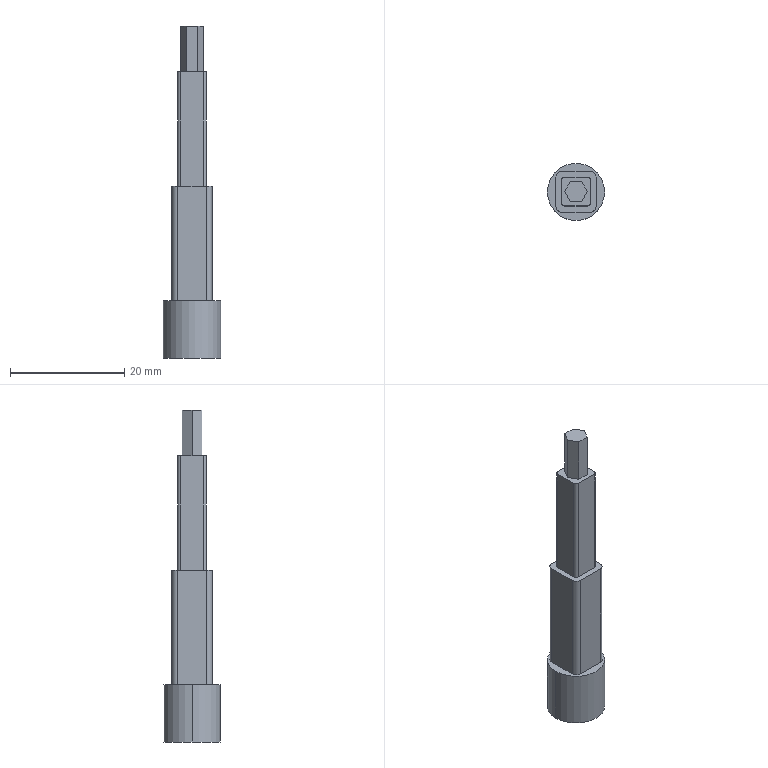Part | SolidWorks | features ICE 3, Fillet 2, Extrusion 1 | 1 solid | 29 faces | box 10 x 10 x 58 mm | volume 2347 mm3 | plane 19 | cylinder 10 | commonest cylinder face diameters 1 x4 2 x4 10 x2
STEP:
#1=CARTESIAN_POINT('',(5.,0.,10.));
#2=VERTEX_POINT('',#1);
#3=CARTESIAN_POINT('',(-5.,0.,10.));
#4=VERTEX_POINT('',#3);
#5=CARTESIAN_POINT('',(0.,0.,10.));
#6=DIRECTION('',(0.,0.,1.));
#7=DIRECTION('',(1.,0.,0.));
#8=AXIS2_PLACEMENT_3D('',#5,#6,#7);
#9=CIRCLE('',#8,5.);
#10=EDGE_CURVE('',#2,#4,#9,.T.);
#11=ORIENTED_EDGE('',*,*,#10,.F.);
#12=CARTESIAN_POINT('',(5.,0.,0.));
#13=VERTEX_POINT('',#12);
#14=CARTESIAN_POINT('',(5.,0.,10.));
#15=DIRECTION('',(0.,0.,-1.));
#16=VECTOR('',#15,1000.);
#17=LINE('',#14,#16);
#18=EDGE_CURVE('',#2,#13,#17,.T.);
#19=ORIENTED_EDGE('',*,*,#18,.T.);
#20=CARTESIAN_POINT('',(-5.,0.,0.));
#21=VERTEX_POINT('',#20);
#22=CARTESIAN_POINT('',(0.,0.,0.));
#23=DIRECTION('',(0.,0.,1.));
#24=DIRECTION('',(1.,0.,0.));
#25=AXIS2_PLACEMENT_3D('',#22,#23,#24);
#26=CIRCLE('',#25,5.);
#27=EDGE_CURVE('',#13,#21,#26,.T.);
#28=ORIENTED_EDGE('',*,*,#27,.T.);
#29=CARTESIAN_POINT('',(-5.,0.,10.));
#30=DIRECTION('',(0.,0.,-1.));
#31=VECTOR('',#30,1000.);
#32=LINE('',#29,#31);
#33=EDGE_CURVE('',#4,#21,#32,.T.);
#34=ORIENTED_EDGE('',*,*,#33,.F.);
#35=EDGE_LOOP('',(#11,#19,#28,#34));
#36=FACE_OUTER_BOUND('',#35,.T.);
#37=CARTESIAN_POINT('',(0.,0.,10.));
#38=DIRECTION('',(0.,0.,-1.));
#39=DIRECTION('',(-1.,0.,0.));
#40=AXIS2_PLACEMENT_3D('',#37,#38,#39);
#41=CYLINDRICAL_SURFACE('',#40,5.);
#42=ADVANCED_FACE('',(#36),#41,.T.);
#43=CARTESIAN_POINT('',(0.,0.,10.));
#44=DIRECTION('',(0.,0.,1.));
#45=DIRECTION('',(1.,0.,0.));
#46=AXIS2_PLACEMENT_3D('',#43,#44,#45);
#47=CIRCLE('',#46,5.);
#48=EDGE_CURVE('',#4,#2,#47,.T.);
#49=ORIENTED_EDGE('',*,*,#48,.T.);
#50=ORIENTED_EDGE('',*,*,#10,.T.);
#51=EDGE_LOOP('',(#49,#50));
#52=FACE_OUTER_BOUND('',#51,.T.);
#53=CARTESIAN_POINT('',(3.5,-2.571,10.));
#54=VERTEX_POINT('',#53);
#55=CARTESIAN_POINT('',(3.5,2.571,10.));
#56=VERTEX_POINT('',#55);
#57=CARTESIAN_POINT('',(3.5,3.571,10.));
#58=DIRECTION('',(0.,1.,0.));
#59=VECTOR('',#58,1000.);
#60=LINE('',#57,#59);
#61=EDGE_CURVE('',#54,#56,#60,.T.);
#62=ORIENTED_EDGE('',*,*,#61,.F.);
#63=CARTESIAN_POINT('',(2.5,-3.571,10.));
#64=VERTEX_POINT('',#63);
#65=CARTESIAN_POINT('',(2.5,-2.571,10.));
#66=DIRECTION('',(0.,0.,-1.));
#67=DIRECTION('',(1.,0.,0.));
#68=AXIS2_PLACEMENT_3D('',#65,#66,#67);
#69=CIRCLE('',#68,1.);
#70=EDGE_CURVE('',#54,#64,#69,.T.);
#71=ORIENTED_EDGE('',*,*,#70,.T.);
#72=CARTESIAN_POINT('',(-2.5,-3.571,10.));
#73=VERTEX_POINT('',#72);
#74=CARTESIAN_POINT('',(-3.5,-3.571,10.));
#75=DIRECTION('',(1.,0.,0.));
#76=VECTOR('',#75,1000.);
#77=LINE('',#74,#76);
#78=EDGE_CURVE('',#73,#64,#77,.T.);
#79=ORIENTED_EDGE('',*,*,#78,.F.);
#80=CARTESIAN_POINT('',(-3.5,-2.571,10.));
#81=VERTEX_POINT('',#80);
#82=CARTESIAN_POINT('',(-2.5,-2.571,10.));
#83=DIRECTION('',(0.,0.,-1.));
#84=DIRECTION('',(1.,0.,0.));
#85=AXIS2_PLACEMENT_3D('',#82,#83,#84);
#86=CIRCLE('',#85,1.);
#87=EDGE_CURVE('',#73,#81,#86,.T.);
#88=ORIENTED_EDGE('',*,*,#87,.T.);
#89=CARTESIAN_POINT('',(-3.5,2.571,10.));
#90=VERTEX_POINT('',#89);
#91=CARTESIAN_POINT('',(-3.5,3.571,10.));
#92=DIRECTION('',(0.,-1.,0.));
#93=VECTOR('',#92,1000.);
#94=LINE('',#91,#93);
#95=EDGE_CURVE('',#90,#81,#94,.T.);
#96=ORIENTED_EDGE('',*,*,#95,.F.);
#97=CARTESIAN_POINT('',(-2.5,3.571,10.));
#98=VERTEX_POINT('',#97);
#99=CARTESIAN_POINT('',(-2.5,2.571,10.));
#100=DIRECTION('',(0.,0.,-1.));
#101=DIRECTION('',(1.,0.,0.));
#102=AXIS2_PLACEMENT_3D('',#99,#100,#101);
#103=CIRCLE('',#102,1.);
#104=EDGE_CURVE('',#90,#98,#103,.T.);
#105=ORIENTED_EDGE('',*,*,#104,.T.);
#106=CARTESIAN_POINT('',(2.5,3.571,10.));
#107=VERTEX_POINT('',#106);
#108=CARTESIAN_POINT('',(-3.5,3.571,10.));
#109=DIRECTION('',(-1.,0.,0.));
#110=VECTOR('',#109,1000.);
#111=LINE('',#108,#110);
#112=EDGE_CURVE('',#107,#98,#111,.T.);
#113=ORIENTED_EDGE('',*,*,#112,.F.);
#114=CARTESIAN_POINT('',(2.5,2.571,10.));
#115=DIRECTION('',(0.,0.,-1.));
#116=DIRECTION('',(1.,0.,0.));
#117=AXIS2_PLACEMENT_3D('',#114,#115,#116);
#118=CIRCLE('',#117,1.);
#119=EDGE_CURVE('',#107,#56,#118,.T.);
#120=ORIENTED_EDGE('',*,*,#119,.T.);
#121=EDGE_LOOP('',(#62,#71,#79,#88,#96,#105,#113,#120));
#122=FACE_BOUND('',#121,.T.);
#123=CARTESIAN_POINT('',(0.,0.,10.));
#124=DIRECTION('',(0.,0.,1.));
#125=DIRECTION('',(1.,0.,0.));
#126=AXIS2_PLACEMENT_3D('',#123,#124,#125);
#127=PLANE('',#126);
#128=ADVANCED_FACE('',(#52,#122),#127,.T.);
#129=ORIENTED_EDGE('',*,*,#18,.F.);
#130=ORIENTED_EDGE('',*,*,#48,.F.);
#131=ORIENTED_EDGE('',*,*,#33,.T.);
#132=CARTESIAN_POINT('',(0.,0.,0.));
#133=DIRECTION('',(0.,0.,1.));
#134=DIRECTION('',(1.,0.,0.));
#135=AXIS2_PLACEMENT_3D('',#132,#133,#134);
#136=CIRCLE('',#135,5.);
#137=EDGE_CURVE('',#21,#13,#136,.T.);
#138=ORIENTED_EDGE('',*,*,#137,.T.);
#139=EDGE_LOOP('',(#129,#130,#131,#138));
#140=FACE_OUTER_BOUND('',#139,.T.);
#141=CARTESIAN_POINT('',(0.,0.,10.));
#142=DIRECTION('',(0.,0.,-1.));
#143=DIRECTION('',(-1.,0.,0.));
#144=AXIS2_PLACEMENT_3D('',#141,#142,#143);
#145=CYLINDRICAL_SURFACE('',#144,5.);
#146=ADVANCED_FACE('',(#140),#145,.T.);
#147=ORIENTED_EDGE('',*,*,#137,.F.);
#148=ORIENTED_EDGE('',*,*,#27,.F.);
#149=EDGE_LOOP('',(#147,#148));
#150=FACE_OUTER_BOUND('',#149,.T.);
#151=CARTESIAN_POINT('',(0.,0.,0.));
#152=DIRECTION('',(0.,0.,1.));
#153=DIRECTION('',(1.,0.,0.));
#154=AXIS2_PLACEMENT_3D('',#151,#152,#153);
#155=PLANE('',#154);
#156=ADVANCED_FACE('',(#150),#155,.F.);
#157=ORIENTED_EDGE('',*,*,#95,.T.);
#158=CARTESIAN_POINT('',(-3.5,-2.571,30.));
#159=VERTEX_POINT('',#158);
#160=CARTESIAN_POINT('',(-3.5,-2.571,30.));
#161=DIRECTION('',(0.,0.,1.));
#162=VECTOR('',#161,1000.);
#163=LINE('',#160,#162);
#164=EDGE_CURVE('',#81,#159,#163,.T.);
#165=ORIENTED_EDGE('',*,*,#164,.T.);
#166=CARTESIAN_POINT('',(-3.5,2.571,30.));
#167=VERTEX_POINT('',#166);
#168=CARTESIAN_POINT('',(-3.5,3.571,30.));
#169=DIRECTION('',(0.,-1.,0.));
#170=VECTOR('',#169,1000.);
#171=LINE('',#168,#170);
#172=EDGE_CURVE('',#167,#159,#171,.T.);
#173=ORIENTED_EDGE('',*,*,#172,.F.);
#174=CARTESIAN_POINT('',(-3.5,2.571,30.));
#175=DIRECTION('',(0.,0.,-1.));
#176=VECTOR('',#175,1000.);
#177=LINE('',#174,#176);
#178=EDGE_CURVE('',#167,#90,#177,.T.);
#179=ORIENTED_EDGE('',*,*,#178,.T.);
#180=EDGE_LOOP('',(#157,#165,#173,#179));
#181=FACE_OUTER_BOUND('',#180,.T.);
#182=CARTESIAN_POINT('',(-3.5,3.571,30.));
#183=DIRECTION('',(1.,0.,0.));
#184=DIRECTION('',(0.,0.,-1.));
#185=AXIS2_PLACEMENT_3D('',#182,#183,#184);
#186=PLANE('',#185);
#187=ADVANCED_FACE('',(#181),#186,.F.);
#188=ORIENTED_EDGE('',*,*,#78,.T.);
#189=CARTESIAN_POINT('',(2.5,-3.571,30.));
#190=VERTEX_POINT('',#189);
#191=CARTESIAN_POINT('',(2.5,-3.571,30.));
#192=DIRECTION('',(0.,0.,1.));
#193=VECTOR('',#192,1000.);
#194=LINE('',#191,#193);
#195=EDGE_CURVE('',#64,#190,#194,.T.);
#196=ORIENTED_EDGE('',*,*,#195,.T.);
#197=CARTESIAN_POINT('',(-2.5,-3.571,30.));
#198=VERTEX_POINT('',#197);
#199=CARTESIAN_POINT('',(-3.5,-3.571,30.));
#200=DIRECTION('',(1.,0.,0.));
#201=VECTOR('',#200,1000.);
#202=LINE('',#199,#201);
#203=EDGE_CURVE('',#198,#190,#202,.T.);
#204=ORIENTED_EDGE('',*,*,#203,.F.);
#205=CARTESIAN_POINT('',(-2.5,-3.571,30.));
#206=DIRECTION('',(0.,0.,-1.));
#207=VECTOR('',#206,1000.);
#208=LINE('',#205,#207);
#209=EDGE_CURVE('',#198,#73,#208,.T.);
#210=ORIENTED_EDGE('',*,*,#209,.T.);
#211=EDGE_LOOP('',(#188,#196,#204,#210));
#212=FACE_OUTER_BOUND('',#211,.T.);
#213=CARTESIAN_POINT('',(-3.5,-3.571,30.));
#214=DIRECTION('',(0.,1.,0.));
#215=DIRECTION('',(0.,0.,1.));
#216=AXIS2_PLACEMENT_3D('',#213,#214,#215);
#217=PLANE('',#216);
#218=ADVANCED_FACE('',(#212),#217,.F.);
#219=CARTESIAN_POINT('',(3.5,-2.571,30.));
#220=VERTEX_POINT('',#219);
#221=CARTESIAN_POINT('',(3.5,2.571,30.));
#222=VERTEX_POINT('',#221);
#223=CARTESIAN_POINT('',(3.5,3.571,30.));
#224=DIRECTION('',(0.,1.,0.));
#225=VECTOR('',#224,1000.);
#226=LINE('',#223,#225);
#227=EDGE_CURVE('',#220,#222,#226,.T.);
#228=ORIENTED_EDGE('',*,*,#227,.F.);
#229=CARTESIAN_POINT('',(3.5,-2.571,30.));
#230=DIRECTION('',(0.,0.,-1.));
#231=VECTOR('',#230,1000.);
#232=LINE('',#229,#231);
#233=EDGE_CURVE('',#220,#54,#232,.T.);
#234=ORIENTED_EDGE('',*,*,#233,.T.);
#235=ORIENTED_EDGE('',*,*,#61,.T.);
#236=CARTESIAN_POINT('',(3.5,2.571,30.));
#237=DIRECTION('',(0.,0.,1.));
#238=VECTOR('',#237,1000.);
#239=LINE('',#236,#238);
#240=EDGE_CURVE('',#56,#222,#239,.T.);
#241=ORIENTED_EDGE('',*,*,#240,.T.);
#242=EDGE_LOOP('',(#228,#234,#235,#241));
#243=FACE_OUTER_BOUND('',#242,.T.);
#244=CARTESIAN_POINT('',(3.5,3.571,30.));
#245=DIRECTION('',(-1.,0.,0.));
#246=DIRECTION('',(0.,0.,1.));
#247=AXIS2_PLACEMENT_3D('',#244,#245,#246);
#248=PLANE('',#247);
#249=ADVANCED_FACE('',(#243),#248,.F.);
#250=ORIENTED_EDGE('',*,*,#112,.T.);
#251=CARTESIAN_POINT('',(-2.5,3.571,30.));
#252=VERTEX_POINT('',#251);
#253=CARTESIAN_POINT('',(-2.5,3.571,30.));
#254=DIRECTION('',(0.,0.,1.));
#255=VECTOR('',#254,1000.);
#256=LINE('',#253,#255);
#257=EDGE_CURVE('',#98,#252,#256,.T.);
#258=ORIENTED_EDGE('',*,*,#257,.T.);
#259=CARTESIAN_POINT('',(2.5,3.571,30.));
#260=VERTEX_POINT('',#259);
#261=CARTESIAN_POINT('',(-3.5,3.571,30.));
#262=DIRECTION('',(-1.,0.,0.));
#263=VECTOR('',#262,1000.);
#264=LINE('',#261,#263);
#265=EDGE_CURVE('',#260,#252,#264,.T.);
#266=ORIENTED_EDGE('',*,*,#265,.F.);
#267=CARTESIAN_POINT('',(2.5,3.571,30.));
#268=DIRECTION('',(0.,0.,-1.));
#269=VECTOR('',#268,1000.);
#270=LINE('',#267,#269);
#271=EDGE_CURVE('',#260,#107,#270,.T.);
#272=ORIENTED_EDGE('',*,*,#271,.T.);
#273=EDGE_LOOP('',(#250,#258,#266,#272));
#274=FACE_OUTER_BOUND('',#273,.T.);
#275=CARTESIAN_POINT('',(-3.5,3.571,30.));
#276=DIRECTION('',(0.,-1.,0.));
#277=DIRECTION('',(0.,0.,-1.));
#278=AXIS2_PLACEMENT_3D('',#275,#276,#277);
#279=PLANE('',#278);
#280=ADVANCED_FACE('',(#274),#279,.F.);
#281=CARTESIAN_POINT('',(-2.5,2.,30.));
#282=VERTEX_POINT('',#281);
#283=CARTESIAN_POINT('',(-2.5,-2.,30.));
#284=VERTEX_POINT('',#283);
#285=CARTESIAN_POINT('',(-2.5,-2.5,30.));
#286=DIRECTION('',(0.,-1.,0.));
#287=VECTOR('',#286,1000.);
#288=LINE('',#285,#287);
#289=EDGE_CURVE('',#282,#284,#288,.T.);
#290=ORIENTED_EDGE('',*,*,#289,.F.);
#291=CARTESIAN_POINT('',(-2.,2.5,30.));
#292=VERTEX_POINT('',#291);
#293=CARTESIAN_POINT('',(-2.,2.,30.));
#294=DIRECTION('',(0.,0.,-1.));
#295=DIRECTION('',(1.,0.,0.));
#296=AXIS2_PLACEMENT_3D('',#293,#294,#295);
#297=CIRCLE('',#296,0.5);
#298=EDGE_CURVE('',#282,#292,#297,.T.);
#299=ORIENTED_EDGE('',*,*,#298,.T.);
#300=CARTESIAN_POINT('',(2.,2.5,30.));
#301=VERTEX_POINT('',#300);
#302=CARTESIAN_POINT('',(2.5,2.5,30.));
#303=DIRECTION('',(-1.,0.,0.));
#304=VECTOR('',#303,1000.);
#305=LINE('',#302,#304);
#306=EDGE_CURVE('',#301,#292,#305,.T.);
#307=ORIENTED_EDGE('',*,*,#306,.F.);
#308=CARTESIAN_POINT('',(2.5,2.,30.));
#309=VERTEX_POINT('',#308);
#310=CARTESIAN_POINT('',(2.,2.,30.));
#311=DIRECTION('',(0.,0.,-1.));
#312=DIRECTION('',(1.,0.,0.));
#313=AXIS2_PLACEMENT_3D('',#310,#311,#312);
#314=CIRCLE('',#313,0.5);
#315=EDGE_CURVE('',#301,#309,#314,.T.);
#316=ORIENTED_EDGE('',*,*,#315,.T.);
#317=CARTESIAN_POINT('',(2.5,-2.,30.));
#318=VERTEX_POINT('',#317);
#319=CARTESIAN_POINT('',(2.5,-2.5,30.));
#320=DIRECTION('',(0.,1.,0.));
#321=VECTOR('',#320,1000.);
#322=LINE('',#319,#321);
#323=EDGE_CURVE('',#318,#309,#322,.T.);
#324=ORIENTED_EDGE('',*,*,#323,.F.);
#325=CARTESIAN_POINT('',(2.,-2.5,30.));
#326=VERTEX_POINT('',#325);
#327=CARTESIAN_POINT('',(2.,-2.,30.));
#328=DIRECTION('',(0.,0.,-1.));
#329=DIRECTION('',(1.,0.,0.));
#330=AXIS2_PLACEMENT_3D('',#327,#328,#329);
#331=CIRCLE('',#330,0.5);
#332=EDGE_CURVE('',#318,#326,#331,.T.);
#333=ORIENTED_EDGE('',*,*,#332,.T.);
#334=CARTESIAN_POINT('',(-2.,-2.5,30.));
#335=VERTEX_POINT('',#334);
#336=CARTESIAN_POINT('',(2.5,-2.5,30.));
#337=DIRECTION('',(1.,0.,0.));
#338=VECTOR('',#337,1000.);
#339=LINE('',#336,#338);
#340=EDGE_CURVE('',#335,#326,#339,.T.);
#341=ORIENTED_EDGE('',*,*,#340,.F.);
#342=CARTESIAN_POINT('',(-2.,-2.,30.));
#343=DIRECTION('',(0.,0.,-1.));
#344=DIRECTION('',(1.,0.,0.));
#345=AXIS2_PLACEMENT_3D('',#342,#343,#344);
#346=CIRCLE('',#345,0.5);
#347=EDGE_CURVE('',#335,#284,#346,.T.);
#348=ORIENTED_EDGE('',*,*,#347,.T.);
#349=EDGE_LOOP('',(#290,#299,#307,#316,#324,#333,#341,#348));
#350=FACE_BOUND('',#349,.T.);
#351=ORIENTED_EDGE('',*,*,#203,.T.);
#352=CARTESIAN_POINT('',(2.5,-2.571,30.));
#353=DIRECTION('',(0.,0.,1.));
#354=DIRECTION('',(1.,0.,0.));
#355=AXIS2_PLACEMENT_3D('',#352,#353,#354);
#356=CIRCLE('',#355,1.);
#357=EDGE_CURVE('',#190,#220,#356,.T.);
#358=ORIENTED_EDGE('',*,*,#357,.T.);
#359=ORIENTED_EDGE('',*,*,#227,.T.);
#360=CARTESIAN_POINT('',(2.5,2.571,30.));
#361=DIRECTION('',(0.,0.,1.));
#362=DIRECTION('',(1.,0.,0.));
#363=AXIS2_PLACEMENT_3D('',#360,#361,#362);
#364=CIRCLE('',#363,1.);
#365=EDGE_CURVE('',#222,#260,#364,.T.);
#366=ORIENTED_EDGE('',*,*,#365,.T.);
#367=ORIENTED_EDGE('',*,*,#265,.T.);
#368=CARTESIAN_POINT('',(-2.5,2.571,30.));
#369=DIRECTION('',(0.,0.,1.));
#370=DIRECTION('',(1.,0.,0.));
#371=AXIS2_PLACEMENT_3D('',#368,#369,#370);
#372=CIRCLE('',#371,1.);
#373=EDGE_CURVE('',#252,#167,#372,.T.);
#374=ORIENTED_EDGE('',*,*,#373,.T.);
#375=ORIENTED_EDGE('',*,*,#172,.T.);
#376=CARTESIAN_POINT('',(-2.5,-2.571,30.));
#377=DIRECTION('',(0.,0.,1.));
#378=DIRECTION('',(1.,0.,0.));
#379=AXIS2_PLACEMENT_3D('',#376,#377,#378);
#380=CIRCLE('',#379,1.);
#381=EDGE_CURVE('',#159,#198,#380,.T.);
#382=ORIENTED_EDGE('',*,*,#381,.T.);
#383=EDGE_LOOP('',(#351,#358,#359,#366,#367,#374,#375,#382));
#384=FACE_OUTER_BOUND('',#383,.T.);
#385=CARTESIAN_POINT('',(0.,0.,30.));
#386=DIRECTION('',(0.,0.,1.));
#387=DIRECTION('',(1.,0.,0.));
#388=AXIS2_PLACEMENT_3D('',#385,#386,#387);
#389=PLANE('',#388);
#390=ADVANCED_FACE('',(#350,#384),#389,.T.);
#391=ORIENTED_EDGE('',*,*,#357,.F.);
#392=ORIENTED_EDGE('',*,*,#195,.F.);
#393=ORIENTED_EDGE('',*,*,#70,.F.);
#394=ORIENTED_EDGE('',*,*,#233,.F.);
#395=EDGE_LOOP('',(#391,#392,#393,#394));
#396=FACE_OUTER_BOUND('',#395,.T.);
#397=CARTESIAN_POINT('',(2.5,-2.571,30.));
#398=DIRECTION('',(0.,0.,-1.));
#399=DIRECTION('',(-1.,0.,0.));
#400=AXIS2_PLACEMENT_3D('',#397,#398,#399);
#401=CYLINDRICAL_SURFACE('',#400,1.);
#402=ADVANCED_FACE('',(#396),#401,.T.);
#403=ORIENTED_EDGE('',*,*,#381,.F.);
#404=ORIENTED_EDGE('',*,*,#164,.F.);
#405=ORIENTED_EDGE('',*,*,#87,.F.);
#406=ORIENTED_EDGE('',*,*,#209,.F.);
#407=EDGE_LOOP('',(#403,#404,#405,#406));
#408=FACE_OUTER_BOUND('',#407,.T.);
#409=CARTESIAN_POINT('',(-2.5,-2.571,30.));
#410=DIRECTION('',(0.,0.,-1.));
#411=DIRECTION('',(-1.,0.,0.));
#412=AXIS2_PLACEMENT_3D('',#409,#410,#411);
#413=CYLINDRICAL_SURFACE('',#412,1.);
#414=ADVANCED_FACE('',(#408),#413,.T.);
#415=ORIENTED_EDGE('',*,*,#373,.F.);
#416=ORIENTED_EDGE('',*,*,#257,.F.);
#417=ORIENTED_EDGE('',*,*,#104,.F.);
#418=ORIENTED_EDGE('',*,*,#178,.F.);
#419=EDGE_LOOP('',(#415,#416,#417,#418));
#420=FACE_OUTER_BOUND('',#419,.T.);
#421=CARTESIAN_POINT('',(-2.5,2.571,30.));
#422=DIRECTION('',(0.,0.,-1.));
#423=DIRECTION('',(-1.,0.,0.));
#424=AXIS2_PLACEMENT_3D('',#421,#422,#423);
#425=CYLINDRICAL_SURFACE('',#424,1.);
#426=ADVANCED_FACE('',(#420),#425,.T.);
#427=ORIENTED_EDGE('',*,*,#365,.F.);
#428=ORIENTED_EDGE('',*,*,#240,.F.);
#429=ORIENTED_EDGE('',*,*,#119,.F.);
#430=ORIENTED_EDGE('',*,*,#271,.F.);
#431=EDGE_LOOP('',(#427,#428,#429,#430));
#432=FACE_OUTER_BOUND('',#431,.T.);
#433=CARTESIAN_POINT('',(2.5,2.571,30.));
#434=DIRECTION('',(0.,0.,-1.));
#435=DIRECTION('',(-1.,0.,0.));
#436=AXIS2_PLACEMENT_3D('',#433,#434,#435);
#437=CYLINDRICAL_SURFACE('',#436,1.);
#438=ADVANCED_FACE('',(#432),#437,.T.);
#439=ORIENTED_EDGE('',*,*,#289,.T.);
#440=CARTESIAN_POINT('',(-2.5,-2.,50.));
#441=VERTEX_POINT('',#440);
#442=CARTESIAN_POINT('',(-2.5,-2.,50.));
#443=DIRECTION('',(0.,0.,1.));
#444=VECTOR('',#443,1000.);
#445=LINE('',#442,#444);
#446=EDGE_CURVE('',#284,#441,#445,.T.);
#447=ORIENTED_EDGE('',*,*,#446,.T.);
#448=CARTESIAN_POINT('',(-2.5,2.,50.));
#449=VERTEX_POINT('',#448);
#450=CARTESIAN_POINT('',(-2.5,-2.5,50.));
#451=DIRECTION('',(0.,-1.,0.));
#452=VECTOR('',#451,1000.);
#453=LINE('',#450,#452);
#454=EDGE_CURVE('',#449,#441,#453,.T.);
#455=ORIENTED_EDGE('',*,*,#454,.F.);
#456=CARTESIAN_POINT('',(-2.5,2.,50.));
#457=DIRECTION('',(0.,0.,-1.));
#458=VECTOR('',#457,1000.);
#459=LINE('',#456,#458);
#460=EDGE_CURVE('',#449,#282,#459,.T.);
#461=ORIENTED_EDGE('',*,*,#460,.T.);
#462=EDGE_LOOP('',(#439,#447,#455,#461));
#463=FACE_OUTER_BOUND('',#462,.T.);
#464=CARTESIAN_POINT('',(-2.5,-2.5,50.));
#465=DIRECTION('',(1.,0.,0.));
#466=DIRECTION('',(0.,0.,-1.));
#467=AXIS2_PLACEMENT_3D('',#464,#465,#466);
#468=PLANE('',#467);
#469=ADVANCED_FACE('',(#463),#468,.F.);
#470=ORIENTED_EDGE('',*,*,#340,.T.);
#471=CARTESIAN_POINT('',(2.,-2.5,50.));
#472=VERTEX_POINT('',#471);
#473=CARTESIAN_POINT('',(2.,-2.5,50.));
#474=DIRECTION('',(0.,0.,1.));
#475=VECTOR('',#474,1000.);
#476=LINE('',#473,#475);
#477=EDGE_CURVE('',#326,#472,#476,.T.);
#478=ORIENTED_EDGE('',*,*,#477,.T.);
#479=CARTESIAN_POINT('',(-2.,-2.5,50.));
#480=VERTEX_POINT('',#479);
#481=CARTESIAN_POINT('',(2.5,-2.5,50.));
#482=DIRECTION('',(1.,0.,0.));
#483=VECTOR('',#482,1000.);
#484=LINE('',#481,#483);
#485=EDGE_CURVE('',#480,#472,#484,.T.);
#486=ORIENTED_EDGE('',*,*,#485,.F.);
#487=CARTESIAN_POINT('',(-2.,-2.5,50.));
#488=DIRECTION('',(0.,0.,-1.));
#489=VECTOR('',#488,1000.);
#490=LINE('',#487,#489);
#491=EDGE_CURVE('',#480,#335,#490,.T.);
#492=ORIENTED_EDGE('',*,*,#491,.T.);
#493=EDGE_LOOP('',(#470,#478,#486,#492));
#494=FACE_OUTER_BOUND('',#493,.T.);
#495=CARTESIAN_POINT('',(2.5,-2.5,50.));
#496=DIRECTION('',(0.,1.,0.));
#497=DIRECTION('',(-1.,0.,0.));
#498=AXIS2_PLACEMENT_3D('',#495,#496,#497);
#499=PLANE('',#498);
#500=ADVANCED_FACE('',(#494),#499,.F.);
#501=CARTESIAN_POINT('',(2.5,-2.,50.));
#502=VERTEX_POINT('',#501);
#503=CARTESIAN_POINT('',(2.5,2.,50.));
#504=VERTEX_POINT('',#503);
#505=CARTESIAN_POINT('',(2.5,-2.5,50.));
#506=DIRECTION('',(0.,1.,0.));
#507=VECTOR('',#506,1000.);
#508=LINE('',#505,#507);
#509=EDGE_CURVE('',#502,#504,#508,.T.);
#510=ORIENTED_EDGE('',*,*,#509,.F.);
#511=CARTESIAN_POINT('',(2.5,-2.,50.));
#512=DIRECTION('',(0.,0.,-1.));
#513=VECTOR('',#512,1000.);
#514=LINE('',#511,#513);
#515=EDGE_CURVE('',#502,#318,#514,.T.);
#516=ORIENTED_EDGE('',*,*,#515,.T.);
#517=ORIENTED_EDGE('',*,*,#323,.T.);
#518=CARTESIAN_POINT('',(2.5,2.,50.));
#519=DIRECTION('',(0.,0.,1.));
#520=VECTOR('',#519,1000.);
#521=LINE('',#518,#520);
#522=EDGE_CURVE('',#309,#504,#521,.T.);
#523=ORIENTED_EDGE('',*,*,#522,.T.);
#524=EDGE_LOOP('',(#510,#516,#517,#523));
#525=FACE_OUTER_BOUND('',#524,.T.);
#526=CARTESIAN_POINT('',(2.5,-2.5,50.));
#527=DIRECTION('',(-1.,0.,0.));
#528=DIRECTION('',(0.,0.,1.));
#529=AXIS2_PLACEMENT_3D('',#526,#527,#528);
#530=PLANE('',#529);
#531=ADVANCED_FACE('',(#525),#530,.F.);
#532=ORIENTED_EDGE('',*,*,#306,.T.);
#533=CARTESIAN_POINT('',(-2.,2.5,50.));
#534=VERTEX_POINT('',#533);
#535=CARTESIAN_POINT('',(-2.,2.5,50.));
#536=DIRECTION('',(0.,0.,1.));
#537=VECTOR('',#536,1000.);
#538=LINE('',#535,#537);
#539=EDGE_CURVE('',#292,#534,#538,.T.);
#540=ORIENTED_EDGE('',*,*,#539,.T.);
#541=CARTESIAN_POINT('',(2.,2.5,50.));
#542=VERTEX_POINT('',#541);
#543=CARTESIAN_POINT('',(2.5,2.5,50.));
#544=DIRECTION('',(-1.,0.,0.));
#545=VECTOR('',#544,1000.);
#546=LINE('',#543,#545);
#547=EDGE_CURVE('',#542,#534,#546,.T.);
#548=ORIENTED_EDGE('',*,*,#547,.F.);
#549=CARTESIAN_POINT('',(2.,2.5,50.));
#550=DIRECTION('',(0.,0.,-1.));
#551=VECTOR('',#550,1000.);
#552=LINE('',#549,#551);
#553=EDGE_CURVE('',#542,#301,#552,.T.);
#554=ORIENTED_EDGE('',*,*,#553,.T.);
#555=EDGE_LOOP('',(#532,#540,#548,#554));
#556=FACE_OUTER_BOUND('',#555,.T.);
#557=CARTESIAN_POINT('',(2.5,2.5,50.));
#558=DIRECTION('',(0.,-1.,0.));
#559=DIRECTION('',(0.,0.,-1.));
#560=AXIS2_PLACEMENT_3D('',#557,#558,#559);
#561=PLANE('',#560);
#562=ADVANCED_FACE('',(#556),#561,.F.);
#563=CARTESIAN_POINT('',(2.,0.,50.));
#564=VERTEX_POINT('',#563);
#565=CARTESIAN_POINT('',(1.,1.732,50.));
#566=VERTEX_POINT('',#565);
#567=CARTESIAN_POINT('',(2.,0.,50.));
#568=DIRECTION('',(-0.5,0.866,0.));
#569=VECTOR('',#568,1000.);
#570=LINE('',#567,#569);
#571=EDGE_CURVE('',#564,#566,#570,.T.);
#572=ORIENTED_EDGE('',*,*,#571,.F.);
#573=CARTESIAN_POINT('',(1.,-1.732,50.));
#574=VERTEX_POINT('',#573);
#575=CARTESIAN_POINT('',(1.,-1.732,50.));
#576=DIRECTION('',(0.5,0.866,0.));
#577=VECTOR('',#576,1000.);
#578=LINE('',#575,#577);
#579=EDGE_CURVE('',#574,#564,#578,.T.);
#580=ORIENTED_EDGE('',*,*,#579,.F.);
#581=CARTESIAN_POINT('',(-1.,-1.732,50.));
#582=VERTEX_POINT('',#581);
#583=CARTESIAN_POINT('',(-1.,-1.732,50.));
#584=DIRECTION('',(1.,0.,0.));
#585=VECTOR('',#584,1000.);
#586=LINE('',#583,#585);
#587=EDGE_CURVE('',#582,#574,#586,.T.);
#588=ORIENTED_EDGE('',*,*,#587,.F.);
#589=CARTESIAN_POINT('',(-2.,0.,50.));
#590=VERTEX_POINT('',#589);
#591=CARTESIAN_POINT('',(-2.,0.,50.));
#592=DIRECTION('',(0.5,-0.866,0.));
#593=VECTOR('',#592,1000.);
#594=LINE('',#591,#593);
#595=EDGE_CURVE('',#590,#582,#594,.T.);
#596=ORIENTED_EDGE('',*,*,#595,.F.);
#597=CARTESIAN_POINT('',(-1.,1.732,50.));
#598=VERTEX_POINT('',#597);
#599=CARTESIAN_POINT('',(-1.,1.732,50.));
#600=DIRECTION('',(-0.5,-0.866,0.));
#601=VECTOR('',#600,1000.);
#602=LINE('',#599,#601);
#603=EDGE_CURVE('',#598,#590,#602,.T.);
#604=ORIENTED_EDGE('',*,*,#603,.F.);
#605=CARTESIAN_POINT('',(1.,1.732,50.));
#606=DIRECTION('',(-1.,0.,0.));
#607=VECTOR('',#606,1000.);
#608=LINE('',#605,#607);
#609=EDGE_CURVE('',#566,#598,#608,.T.);
#610=ORIENTED_EDGE('',*,*,#609,.F.);
#611=EDGE_LOOP('',(#572,#580,#588,#596,#604,#610));
#612=FACE_BOUND('',#611,.T.);
#613=ORIENTED_EDGE('',*,*,#485,.T.);
#614=CARTESIAN_POINT('',(2.,-2.,50.));
#615=DIRECTION('',(0.,0.,1.));
#616=DIRECTION('',(1.,0.,0.));
#617=AXIS2_PLACEMENT_3D('',#614,#615,#616);
#618=CIRCLE('',#617,0.5);
#619=EDGE_CURVE('',#472,#502,#618,.T.);
#620=ORIENTED_EDGE('',*,*,#619,.T.);
#621=ORIENTED_EDGE('',*,*,#509,.T.);
#622=CARTESIAN_POINT('',(2.,2.,50.));
#623=DIRECTION('',(0.,0.,1.));
#624=DIRECTION('',(1.,0.,0.));
#625=AXIS2_PLACEMENT_3D('',#622,#623,#624);
#626=CIRCLE('',#625,0.5);
#627=EDGE_CURVE('',#504,#542,#626,.T.);
#628=ORIENTED_EDGE('',*,*,#627,.T.);
#629=ORIENTED_EDGE('',*,*,#547,.T.);
#630=CARTESIAN_POINT('',(-2.,2.,50.));
#631=DIRECTION('',(0.,0.,1.));
#632=DIRECTION('',(1.,0.,0.));
#633=AXIS2_PLACEMENT_3D('',#630,#631,#632);
#634=CIRCLE('',#633,0.5);
#635=EDGE_CURVE('',#534,#449,#634,.T.);
#636=ORIENTED_EDGE('',*,*,#635,.T.);
#637=ORIENTED_EDGE('',*,*,#454,.T.);
#638=CARTESIAN_POINT('',(-2.,-2.,50.));
#639=DIRECTION('',(0.,0.,1.));
#640=DIRECTION('',(1.,0.,0.));
#641=AXIS2_PLACEMENT_3D('',#638,#639,#640);
#642=CIRCLE('',#641,0.5);
#643=EDGE_CURVE('',#441,#480,#642,.T.);
#644=ORIENTED_EDGE('',*,*,#643,.T.);
#645=EDGE_LOOP('',(#613,#620,#621,#628,#629,#636,#637,#644));
#646=FACE_OUTER_BOUND('',#645,.T.);
#647=CARTESIAN_POINT('',(0.,0.,50.));
#648=DIRECTION('',(0.,0.,1.));
#649=DIRECTION('',(1.,0.,0.));
#650=AXIS2_PLACEMENT_3D('',#647,#648,#649);
#651=PLANE('',#650);
#652=ADVANCED_FACE('',(#612,#646),#651,.T.);
#653=ORIENTED_EDGE('',*,*,#619,.F.);
#654=ORIENTED_EDGE('',*,*,#477,.F.);
#655=ORIENTED_EDGE('',*,*,#332,.F.);
#656=ORIENTED_EDGE('',*,*,#515,.F.);
#657=EDGE_LOOP('',(#653,#654,#655,#656));
#658=FACE_OUTER_BOUND('',#657,.T.);
#659=CARTESIAN_POINT('',(2.,-2.,50.));
#660=DIRECTION('',(0.,0.,-1.));
#661=DIRECTION('',(-1.,0.,0.));
#662=AXIS2_PLACEMENT_3D('',#659,#660,#661);
#663=CYLINDRICAL_SURFACE('',#662,0.5);
#664=ADVANCED_FACE('',(#658),#663,.T.);
#665=ORIENTED_EDGE('',*,*,#643,.F.);
#666=ORIENTED_EDGE('',*,*,#446,.F.);
#667=ORIENTED_EDGE('',*,*,#347,.F.);
#668=ORIENTED_EDGE('',*,*,#491,.F.);
#669=EDGE_LOOP('',(#665,#666,#667,#668));
#670=FACE_OUTER_BOUND('',#669,.T.);
#671=CARTESIAN_POINT('',(-2.,-2.,50.));
#672=DIRECTION('',(0.,0.,-1.));
#673=DIRECTION('',(-1.,0.,0.));
#674=AXIS2_PLACEMENT_3D('',#671,#672,#673);
#675=CYLINDRICAL_SURFACE('',#674,0.5);
#676=ADVANCED_FACE('',(#670),#675,.T.);
#677=ORIENTED_EDGE('',*,*,#635,.F.);
#678=ORIENTED_EDGE('',*,*,#539,.F.);
#679=ORIENTED_EDGE('',*,*,#298,.F.);
#680=ORIENTED_EDGE('',*,*,#460,.F.);
#681=EDGE_LOOP('',(#677,#678,#679,#680));
#682=FACE_OUTER_BOUND('',#681,.T.);
#683=CARTESIAN_POINT('',(-2.,2.,50.));
#684=DIRECTION('',(0.,0.,-1.));
#685=DIRECTION('',(-1.,0.,0.));
#686=AXIS2_PLACEMENT_3D('',#683,#684,#685);
#687=CYLINDRICAL_SURFACE('',#686,0.5);
#688=ADVANCED_FACE('',(#682),#687,.T.);
#689=ORIENTED_EDGE('',*,*,#627,.F.);
#690=ORIENTED_EDGE('',*,*,#522,.F.);
#691=ORIENTED_EDGE('',*,*,#315,.F.);
#692=ORIENTED_EDGE('',*,*,#553,.F.);
#693=EDGE_LOOP('',(#689,#690,#691,#692));
#694=FACE_OUTER_BOUND('',#693,.T.);
#695=CARTESIAN_POINT('',(2.,2.,50.));
#696=DIRECTION('',(0.,0.,-1.));
#697=DIRECTION('',(-1.,0.,0.));
#698=AXIS2_PLACEMENT_3D('',#695,#696,#697);
#699=CYLINDRICAL_SURFACE('',#698,0.5);
#700=ADVANCED_FACE('',(#694),#699,.T.);
#701=ORIENTED_EDGE('',*,*,#571,.T.);
#702=CARTESIAN_POINT('',(1.,1.732,58.));
#703=VERTEX_POINT('',#702);
#704=CARTESIAN_POINT('',(1.,1.732,58.));
#705=DIRECTION('',(0.,0.,-1.));
#706=VECTOR('',#705,1000.);
#707=LINE('',#704,#706);
#708=EDGE_CURVE('',#703,#566,#707,.T.);
#709=ORIENTED_EDGE('',*,*,#708,.F.);
#710=CARTESIAN_POINT('',(2.,0.,58.));
#711=VERTEX_POINT('',#710);
#712=CARTESIAN_POINT('',(2.,0.,58.));
#713=DIRECTION('',(-0.5,0.866,0.));
#714=VECTOR('',#713,1000.);
#715=LINE('',#712,#714);
#716=EDGE_CURVE('',#711,#703,#715,.T.);
#717=ORIENTED_EDGE('',*,*,#716,.F.);
#718=CARTESIAN_POINT('',(2.,0.,58.));
#719=DIRECTION('',(0.,0.,-1.));
#720=VECTOR('',#719,1000.);
#721=LINE('',#718,#720);
#722=EDGE_CURVE('',#711,#564,#721,.T.);
#723=ORIENTED_EDGE('',*,*,#722,.T.);
#724=EDGE_LOOP('',(#701,#709,#717,#723));
#725=FACE_OUTER_BOUND('',#724,.T.);
#726=CARTESIAN_POINT('',(2.,0.,58.));
#727=DIRECTION('',(-0.866,-0.5,0.));
#728=DIRECTION('',(0.5,-0.866,0.));
#729=AXIS2_PLACEMENT_3D('',#726,#727,#728);
#730=PLANE('',#729);
#731=ADVANCED_FACE('',(#725),#730,.F.);
#732=ORIENTED_EDGE('',*,*,#609,.T.);
#733=CARTESIAN_POINT('',(-1.,1.732,58.));
#734=VERTEX_POINT('',#733);
#735=CARTESIAN_POINT('',(-1.,1.732,58.));
#736=DIRECTION('',(0.,0.,-1.));
#737=VECTOR('',#736,1000.);
#738=LINE('',#735,#737);
#739=EDGE_CURVE('',#734,#598,#738,.T.);
#740=ORIENTED_EDGE('',*,*,#739,.F.);
#741=CARTESIAN_POINT('',(1.,1.732,58.));
#742=DIRECTION('',(-1.,0.,0.));
#743=VECTOR('',#742,1000.);
#744=LINE('',#741,#743);
#745=EDGE_CURVE('',#703,#734,#744,.T.);
#746=ORIENTED_EDGE('',*,*,#745,.F.);
#747=ORIENTED_EDGE('',*,*,#708,.T.);
#748=EDGE_LOOP('',(#732,#740,#746,#747));
#749=FACE_OUTER_BOUND('',#748,.T.);
#750=CARTESIAN_POINT('',(1.,1.732,58.));
#751=DIRECTION('',(0.,-1.,0.));
#752=DIRECTION('',(1.,0.,0.));
#753=AXIS2_PLACEMENT_3D('',#750,#751,#752);
#754=PLANE('',#753);
#755=ADVANCED_FACE('',(#749),#754,.F.);
#756=ORIENTED_EDGE('',*,*,#603,.T.);
#757=CARTESIAN_POINT('',(-2.,0.,58.));
#758=VERTEX_POINT('',#757);
#759=CARTESIAN_POINT('',(-2.,0.,58.));
#760=DIRECTION('',(0.,0.,-1.));
#761=VECTOR('',#760,1000.);
#762=LINE('',#759,#761);
#763=EDGE_CURVE('',#758,#590,#762,.T.);
#764=ORIENTED_EDGE('',*,*,#763,.F.);
#765=CARTESIAN_POINT('',(-1.,1.732,58.));
#766=DIRECTION('',(-0.5,-0.866,0.));
#767=VECTOR('',#766,1000.);
#768=LINE('',#765,#767);
#769=EDGE_CURVE('',#734,#758,#768,.T.);
#770=ORIENTED_EDGE('',*,*,#769,.F.);
#771=ORIENTED_EDGE('',*,*,#739,.T.);
#772=EDGE_LOOP('',(#756,#764,#770,#771));
#773=FACE_OUTER_BOUND('',#772,.T.);
#774=CARTESIAN_POINT('',(-1.,1.732,58.));
#775=DIRECTION('',(0.866,-0.5,0.));
#776=DIRECTION('',(0.5,0.866,0.));
#777=AXIS2_PLACEMENT_3D('',#774,#775,#776);
#778=PLANE('',#777);
#779=ADVANCED_FACE('',(#773),#778,.F.);
#780=ORIENTED_EDGE('',*,*,#595,.T.);
#781=CARTESIAN_POINT('',(-1.,-1.732,58.));
#782=VERTEX_POINT('',#781);
#783=CARTESIAN_POINT('',(-1.,-1.732,58.));
#784=DIRECTION('',(0.,0.,-1.));
#785=VECTOR('',#784,1000.);
#786=LINE('',#783,#785);
#787=EDGE_CURVE('',#782,#582,#786,.T.);
#788=ORIENTED_EDGE('',*,*,#787,.F.);
#789=CARTESIAN_POINT('',(-2.,0.,58.));
#790=DIRECTION('',(0.5,-0.866,0.));
#791=VECTOR('',#790,1000.);
#792=LINE('',#789,#791);
#793=EDGE_CURVE('',#758,#782,#792,.T.);
#794=ORIENTED_EDGE('',*,*,#793,.F.);
#795=ORIENTED_EDGE('',*,*,#763,.T.);
#796=EDGE_LOOP('',(#780,#788,#794,#795));
#797=FACE_OUTER_BOUND('',#796,.T.);
#798=CARTESIAN_POINT('',(-2.,0.,58.));
#799=DIRECTION('',(0.866,0.5,0.));
#800=DIRECTION('',(-0.5,0.866,0.));
#801=AXIS2_PLACEMENT_3D('',#798,#799,#800);
#802=PLANE('',#801);
#803=ADVANCED_FACE('',(#797),#802,.F.);
#804=ORIENTED_EDGE('',*,*,#587,.T.);
#805=CARTESIAN_POINT('',(1.,-1.732,58.));
#806=VERTEX_POINT('',#805);
#807=CARTESIAN_POINT('',(1.,-1.732,58.));
#808=DIRECTION('',(0.,0.,-1.));
#809=VECTOR('',#808,1000.);
#810=LINE('',#807,#809);
#811=EDGE_CURVE('',#806,#574,#810,.T.);
#812=ORIENTED_EDGE('',*,*,#811,.F.);
#813=CARTESIAN_POINT('',(-1.,-1.732,58.));
#814=DIRECTION('',(1.,0.,0.));
#815=VECTOR('',#814,1000.);
#816=LINE('',#813,#815);
#817=EDGE_CURVE('',#782,#806,#816,.T.);
#818=ORIENTED_EDGE('',*,*,#817,.F.);
#819=ORIENTED_EDGE('',*,*,#787,.T.);
#820=EDGE_LOOP('',(#804,#812,#818,#819));
#821=FACE_OUTER_BOUND('',#820,.T.);
#822=CARTESIAN_POINT('',(-1.,-1.732,58.));
#823=DIRECTION('',(0.,1.,0.));
#824=DIRECTION('',(-1.,0.,0.));
#825=AXIS2_PLACEMENT_3D('',#822,#823,#824);
#826=PLANE('',#825);
#827=ADVANCED_FACE('',(#821),#826,.F.);
#828=ORIENTED_EDGE('',*,*,#579,.T.);
#829=ORIENTED_EDGE('',*,*,#722,.F.);
#830=CARTESIAN_POINT('',(1.,-1.732,58.));
#831=DIRECTION('',(0.5,0.866,0.));
#832=VECTOR('',#831,1000.);
#833=LINE('',#830,#832);
#834=EDGE_CURVE('',#806,#711,#833,.T.);
#835=ORIENTED_EDGE('',*,*,#834,.F.);
#836=ORIENTED_EDGE('',*,*,#811,.T.);
#837=EDGE_LOOP('',(#828,#829,#835,#836));
#838=FACE_OUTER_BOUND('',#837,.T.);
#839=CARTESIAN_POINT('',(1.,-1.732,58.));
#840=DIRECTION('',(-0.866,0.5,0.));
#841=DIRECTION('',(-0.5,-0.866,0.));
#842=AXIS2_PLACEMENT_3D('',#839,#840,#841);
#843=PLANE('',#842);
#844=ADVANCED_FACE('',(#838),#843,.F.);
#845=ORIENTED_EDGE('',*,*,#716,.T.);
#846=ORIENTED_EDGE('',*,*,#745,.T.);
#847=ORIENTED_EDGE('',*,*,#769,.T.);
#848=ORIENTED_EDGE('',*,*,#793,.T.);
#849=ORIENTED_EDGE('',*,*,#817,.T.);
#850=ORIENTED_EDGE('',*,*,#834,.T.);
#851=EDGE_LOOP('',(#845,#846,#847,#848,#849,#850));
#852=FACE_OUTER_BOUND('',#851,.T.);
#853=CARTESIAN_POINT('',(0.,0.,58.));
#854=DIRECTION('',(0.,0.,1.));
#855=DIRECTION('',(1.,0.,0.));
#856=AXIS2_PLACEMENT_3D('',#853,#854,#855);
#857=PLANE('',#856);
#858=ADVANCED_FACE('',(#852),#857,.T.);
#859=CLOSED_SHELL('',(#42,#128,#146,#156,#187,#218,#249,#280,#390,#402,#414,#426,#438,#469,#500,#531,#562,#652,#664,#676,#688,#700,#731,#755,#779,#803,#827,#844,#858));
#860=MANIFOLD_SOLID_BREP('',#859);
#861=CARTESIAN_POINT('',(0.,0.,0.));
#862=DIRECTION('',(0.,0.,1.));
#863=DIRECTION('',(1.,0.,0.));
#864=AXIS2_PLACEMENT_3D('',#861,#862,#863);
#865=(LENGTH_UNIT()NAMED_UNIT(*)SI_UNIT(.MILLI.,.METRE.));
#866=UNCERTAINTY_MEASURE_WITH_UNIT(LENGTH_MEASURE(0.00001),#865,'','');
#867=(NAMED_UNIT(*)PLANE_ANGLE_UNIT()SI_UNIT($,.RADIAN.));
#868=(NAMED_UNIT(*)SI_UNIT($,.STERADIAN.)SOLID_ANGLE_UNIT());
#869=(GEOMETRIC_REPRESENTATION_CONTEXT(3)GLOBAL_UNCERTAINTY_ASSIGNED_CONTEXT((#866))GLOBAL_UNIT_ASSIGNED_CONTEXT((#865,#867,#868))REPRESENTATION_CONTEXT('',''));
#870=ADVANCED_BREP_SHAPE_REPRESENTATION('',(#860,#864),#869);